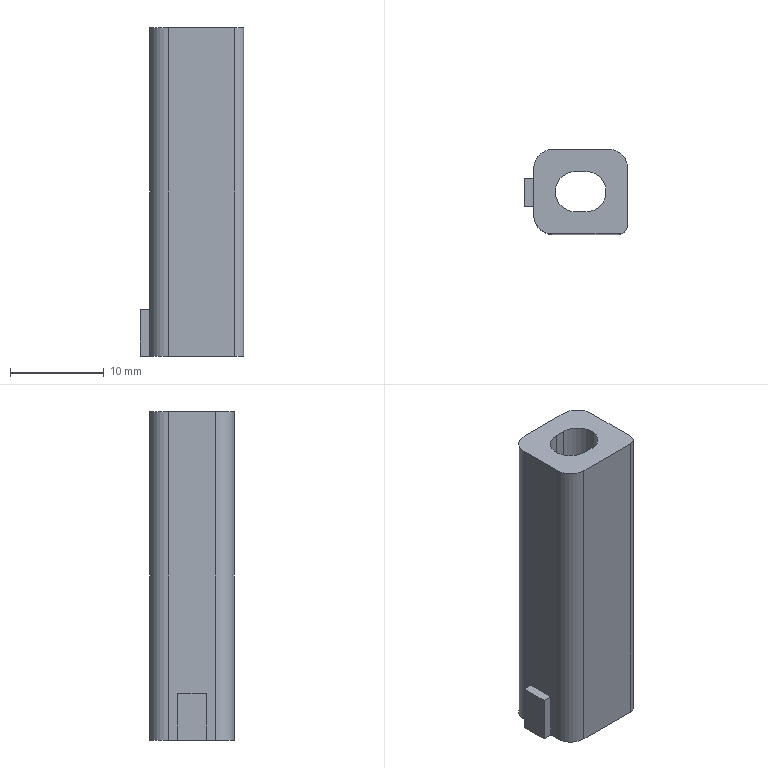Part | NX | features DIE-93 2 | 1 solid | 23 faces | box 11 x 9 x 35 mm | volume 2128 mm3 | plane 15 | cylinder 8 | commonest cylinder face diameters 4 x3 4.32 x2 5.32 x2 2 x1
STEP:
#1=CARTESIAN_POINT('',(4116.686,-879.282,853.716));
#2=VERTEX_POINT('',#1);
#3=CARTESIAN_POINT('',(4117.786,-879.282,853.716));
#4=VERTEX_POINT('',#3);
#5=CARTESIAN_POINT('',(4116.576,-879.282,853.716));
#6=DIRECTION('',(1.,0.,0.));
#7=VECTOR('',#6,1000.);
#8=LINE('',#5,#7);
#9=EDGE_CURVE('',#2,#4,#8,.T.);
#10=ORIENTED_EDGE('',*,*,#9,.F.);
#11=CARTESIAN_POINT('',(4116.686,-879.282,858.716));
#12=VERTEX_POINT('',#11);
#13=CARTESIAN_POINT('',(4116.686,-879.282,862.216));
#14=DIRECTION('',(0.,0.,-1.));
#15=VECTOR('',#14,1000.);
#16=LINE('',#13,#15);
#17=EDGE_CURVE('',#12,#2,#16,.T.);
#18=ORIENTED_EDGE('',*,*,#17,.F.);
#19=CARTESIAN_POINT('',(4117.786,-879.282,858.716));
#20=VERTEX_POINT('',#19);
#21=CARTESIAN_POINT('',(4123.586,-879.282,858.716));
#22=DIRECTION('',(-1.,0.,0.));
#23=VECTOR('',#22,1000.);
#24=LINE('',#21,#23);
#25=EDGE_CURVE('',#20,#12,#24,.T.);
#26=ORIENTED_EDGE('',*,*,#25,.F.);
#27=CARTESIAN_POINT('',(4117.786,-879.282,862.216));
#28=DIRECTION('',(0.,0.,-1.));
#29=VECTOR('',#28,1000.);
#30=LINE('',#27,#29);
#31=EDGE_CURVE('',#4,#20,#30,.F.);
#32=ORIENTED_EDGE('',*,*,#31,.F.);
#33=EDGE_LOOP('',(#10,#18,#26,#32));
#34=FACE_BOUND('',#33,.T.);
#35=CARTESIAN_POINT('',(4116.576,-879.282,870.016));
#36=DIRECTION('',(0.,1.,0.));
#37=DIRECTION('',(1.,0.,0.));
#38=AXIS2_PLACEMENT_3D('',#35,#36,#37);
#39=PLANE('',#38);
#40=ADVANCED_FACE('',(#34),#39,.T.);
#41=CARTESIAN_POINT('',(4117.786,-874.962,858.716));
#42=VERTEX_POINT('',#41);
#43=CARTESIAN_POINT('',(4117.786,-874.962,853.716));
#44=VERTEX_POINT('',#43);
#45=CARTESIAN_POINT('',(4117.786,-874.962,862.216));
#46=DIRECTION('',(0.,0.,-1.));
#47=VECTOR('',#46,1000.);
#48=LINE('',#45,#47);
#49=EDGE_CURVE('',#42,#44,#48,.T.);
#50=ORIENTED_EDGE('',*,*,#49,.T.);
#51=CARTESIAN_POINT('',(4117.786,-877.122,853.716));
#52=DIRECTION('',(0.,0.,1.));
#53=DIRECTION('',(1.,0.,0.));
#54=AXIS2_PLACEMENT_3D('',#51,#52,#53);
#55=CIRCLE('',#54,2.16);
#56=EDGE_CURVE('',#4,#44,#55,.T.);
#57=ORIENTED_EDGE('',*,*,#56,.F.);
#58=ORIENTED_EDGE('',*,*,#31,.T.);
#59=CARTESIAN_POINT('',(4117.786,-877.122,858.716));
#60=DIRECTION('',(0.,0.,1.));
#61=DIRECTION('',(1.,0.,0.));
#62=AXIS2_PLACEMENT_3D('',#59,#60,#61);
#63=CIRCLE('',#62,2.16);
#64=EDGE_CURVE('',#20,#42,#63,.T.);
#65=ORIENTED_EDGE('',*,*,#64,.T.);
#66=EDGE_LOOP('',(#50,#57,#58,#65));
#67=FACE_BOUND('',#66,.T.);
#68=CARTESIAN_POINT('',(4117.786,-877.122,862.216));
#69=DIRECTION('',(0.,0.,-1.));
#70=DIRECTION('',(-1.,0.,0.));
#71=AXIS2_PLACEMENT_3D('',#68,#69,#70);
#72=CYLINDRICAL_SURFACE('',#71,2.16);
#73=ADVANCED_FACE('',(#67),#72,.F.);
#74=CARTESIAN_POINT('',(4116.686,-874.962,853.716));
#75=VERTEX_POINT('',#74);
#76=CARTESIAN_POINT('',(4117.896,-874.962,853.716));
#77=DIRECTION('',(-1.,0.,0.));
#78=VECTOR('',#77,1000.);
#79=LINE('',#76,#78);
#80=EDGE_CURVE('',#44,#75,#79,.T.);
#81=ORIENTED_EDGE('',*,*,#80,.F.);
#82=ORIENTED_EDGE('',*,*,#49,.F.);
#83=CARTESIAN_POINT('',(4116.686,-874.962,858.716));
#84=VERTEX_POINT('',#83);
#85=CARTESIAN_POINT('',(4123.586,-874.962,858.716));
#86=DIRECTION('',(1.,0.,0.));
#87=VECTOR('',#86,1000.);
#88=LINE('',#85,#87);
#89=EDGE_CURVE('',#84,#42,#88,.T.);
#90=ORIENTED_EDGE('',*,*,#89,.F.);
#91=CARTESIAN_POINT('',(4116.686,-874.962,862.216));
#92=DIRECTION('',(0.,0.,-1.));
#93=VECTOR('',#92,1000.);
#94=LINE('',#91,#93);
#95=EDGE_CURVE('',#75,#84,#94,.F.);
#96=ORIENTED_EDGE('',*,*,#95,.F.);
#97=EDGE_LOOP('',(#81,#82,#90,#96));
#98=FACE_BOUND('',#97,.T.);
#99=CARTESIAN_POINT('',(4117.896,-874.962,870.016));
#100=DIRECTION('',(0.,-1.,0.));
#101=DIRECTION('',(-1.,0.,0.));
#102=AXIS2_PLACEMENT_3D('',#99,#100,#101);
#103=PLANE('',#102);
#104=ADVANCED_FACE('',(#98),#103,.T.);
#105=ORIENTED_EDGE('',*,*,#17,.T.);
#106=CARTESIAN_POINT('',(4116.686,-877.122,853.716));
#107=DIRECTION('',(0.,0.,1.));
#108=DIRECTION('',(1.,0.,0.));
#109=AXIS2_PLACEMENT_3D('',#106,#107,#108);
#110=CIRCLE('',#109,2.16);
#111=EDGE_CURVE('',#75,#2,#110,.T.);
#112=ORIENTED_EDGE('',*,*,#111,.F.);
#113=ORIENTED_EDGE('',*,*,#95,.T.);
#114=CARTESIAN_POINT('',(4116.686,-877.122,858.716));
#115=DIRECTION('',(0.,0.,1.));
#116=DIRECTION('',(1.,0.,0.));
#117=AXIS2_PLACEMENT_3D('',#114,#115,#116);
#118=CIRCLE('',#117,2.16);
#119=EDGE_CURVE('',#84,#12,#118,.T.);
#120=ORIENTED_EDGE('',*,*,#119,.T.);
#121=EDGE_LOOP('',(#105,#112,#113,#120));
#122=FACE_BOUND('',#121,.T.);
#123=CARTESIAN_POINT('',(4116.686,-877.122,862.216));
#124=DIRECTION('',(0.,0.,-1.));
#125=DIRECTION('',(1.,0.,0.));
#126=AXIS2_PLACEMENT_3D('',#123,#124,#125);
#127=CYLINDRICAL_SURFACE('',#126,2.16);
#128=ADVANCED_FACE('',(#122),#127,.F.);
#129=ORIENTED_EDGE('',*,*,#119,.F.);
#130=ORIENTED_EDGE('',*,*,#89,.T.);
#131=ORIENTED_EDGE('',*,*,#64,.F.);
#132=ORIENTED_EDGE('',*,*,#25,.T.);
#133=EDGE_LOOP('',(#129,#130,#131,#132));
#134=FACE_BOUND('',#133,.T.);
#135=CARTESIAN_POINT('',(4122.236,-874.622,858.716));
#136=VERTEX_POINT('',#135);
#137=CARTESIAN_POINT('',(4122.236,-880.622,858.716));
#138=VERTEX_POINT('',#137);
#139=CARTESIAN_POINT('',(4122.236,-877.122,858.716));
#140=DIRECTION('',(0.,-1.,0.));
#141=VECTOR('',#140,1000.);
#142=LINE('',#139,#141);
#143=EDGE_CURVE('',#136,#138,#142,.T.);
#144=ORIENTED_EDGE('',*,*,#143,.F.);
#145=CARTESIAN_POINT('',(4120.236,-872.622,858.716));
#146=VERTEX_POINT('',#145);
#147=CARTESIAN_POINT('',(4120.236,-874.622,858.716));
#148=DIRECTION('',(0.,0.,1.));
#149=DIRECTION('',(1.,0.,0.));
#150=AXIS2_PLACEMENT_3D('',#147,#148,#149);
#151=CIRCLE('',#150,2.);
#152=EDGE_CURVE('',#146,#136,#151,.F.);
#153=ORIENTED_EDGE('',*,*,#152,.F.);
#154=CARTESIAN_POINT('',(4114.236,-872.622,858.716));
#155=VERTEX_POINT('',#154);
#156=CARTESIAN_POINT('',(4117.236,-872.622,858.716));
#157=DIRECTION('',(1.,0.,0.));
#158=VECTOR('',#157,1000.);
#159=LINE('',#156,#158);
#160=EDGE_CURVE('',#155,#146,#159,.T.);
#161=ORIENTED_EDGE('',*,*,#160,.F.);
#162=CARTESIAN_POINT('',(4112.236,-874.622,858.716));
#163=VERTEX_POINT('',#162);
#164=CARTESIAN_POINT('',(4114.236,-874.622,858.716));
#165=DIRECTION('',(0.,0.,1.));
#166=DIRECTION('',(1.,0.,0.));
#167=AXIS2_PLACEMENT_3D('',#164,#165,#166);
#168=CIRCLE('',#167,2.);
#169=EDGE_CURVE('',#155,#163,#168,.T.);
#170=ORIENTED_EDGE('',*,*,#169,.T.);
#171=CARTESIAN_POINT('',(4112.236,-879.622,858.716));
#172=VERTEX_POINT('',#171);
#173=CARTESIAN_POINT('',(4112.236,-877.122,858.716));
#174=DIRECTION('',(0.,1.,0.));
#175=VECTOR('',#174,1000.);
#176=LINE('',#173,#175);
#177=EDGE_CURVE('',#172,#163,#176,.T.);
#178=ORIENTED_EDGE('',*,*,#177,.F.);
#179=CARTESIAN_POINT('',(4114.236,-881.622,858.716));
#180=VERTEX_POINT('',#179);
#181=CARTESIAN_POINT('',(4114.236,-879.622,858.716));
#182=DIRECTION('',(0.,0.,1.));
#183=DIRECTION('',(1.,0.,0.));
#184=AXIS2_PLACEMENT_3D('',#181,#182,#183);
#185=CIRCLE('',#184,2.);
#186=EDGE_CURVE('',#172,#180,#185,.T.);
#187=ORIENTED_EDGE('',*,*,#186,.T.);
#188=CARTESIAN_POINT('',(4121.236,-881.622,858.716));
#189=VERTEX_POINT('',#188);
#190=CARTESIAN_POINT('',(4117.236,-881.622,858.716));
#191=DIRECTION('',(-1.,0.,0.));
#192=VECTOR('',#191,1000.);
#193=LINE('',#190,#192);
#194=EDGE_CURVE('',#189,#180,#193,.T.);
#195=ORIENTED_EDGE('',*,*,#194,.F.);
#196=CARTESIAN_POINT('',(4121.236,-880.622,858.716));
#197=DIRECTION('',(0.,0.,1.));
#198=DIRECTION('',(1.,0.,0.));
#199=AXIS2_PLACEMENT_3D('',#196,#197,#198);
#200=CIRCLE('',#199,1.);
#201=EDGE_CURVE('',#138,#189,#200,.F.);
#202=ORIENTED_EDGE('',*,*,#201,.F.);
#203=EDGE_LOOP('',(#144,#153,#161,#170,#178,#187,#195,#202));
#204=FACE_BOUND('',#203,.T.);
#205=CARTESIAN_POINT('',(4123.586,-858.122,858.716));
#206=DIRECTION('',(0.,0.,1.));
#207=DIRECTION('',(-1.,0.,0.));
#208=AXIS2_PLACEMENT_3D('',#205,#206,#207);
#209=PLANE('',#208);
#210=ADVANCED_FACE('',(#134,#204),#209,.T.);
#211=ORIENTED_EDGE('',*,*,#9,.T.);
#212=ORIENTED_EDGE('',*,*,#56,.T.);
#213=ORIENTED_EDGE('',*,*,#80,.T.);
#214=ORIENTED_EDGE('',*,*,#111,.T.);
#215=EDGE_LOOP('',(#211,#212,#213,#214));
#216=FACE_BOUND('',#215,.T.);
#217=CARTESIAN_POINT('',(4117.786,-879.782,853.716));
#218=VERTEX_POINT('',#217);
#219=CARTESIAN_POINT('',(4116.686,-879.782,853.716));
#220=VERTEX_POINT('',#219);
#221=CARTESIAN_POINT('',(4079.736,-879.782,853.716));
#222=DIRECTION('',(-1.,0.,0.));
#223=VECTOR('',#222,1000.);
#224=LINE('',#221,#223);
#225=EDGE_CURVE('',#218,#220,#224,.T.);
#226=ORIENTED_EDGE('',*,*,#225,.T.);
#227=CARTESIAN_POINT('',(4116.686,-874.462,853.716));
#228=VERTEX_POINT('',#227);
#229=CARTESIAN_POINT('',(4116.686,-877.122,853.716));
#230=DIRECTION('',(0.,0.,1.));
#231=DIRECTION('',(1.,0.,0.));
#232=AXIS2_PLACEMENT_3D('',#229,#230,#231);
#233=CIRCLE('',#232,2.66);
#234=EDGE_CURVE('',#220,#228,#233,.F.);
#235=ORIENTED_EDGE('',*,*,#234,.T.);
#236=CARTESIAN_POINT('',(4117.786,-874.462,853.716));
#237=VERTEX_POINT('',#236);
#238=CARTESIAN_POINT('',(4079.736,-874.462,853.716));
#239=DIRECTION('',(1.,0.,0.));
#240=VECTOR('',#239,1000.);
#241=LINE('',#238,#240);
#242=EDGE_CURVE('',#228,#237,#241,.T.);
#243=ORIENTED_EDGE('',*,*,#242,.T.);
#244=CARTESIAN_POINT('',(4117.786,-877.122,853.716));
#245=DIRECTION('',(0.,0.,1.));
#246=DIRECTION('',(1.,0.,0.));
#247=AXIS2_PLACEMENT_3D('',#244,#245,#246);
#248=CIRCLE('',#247,2.66);
#249=EDGE_CURVE('',#237,#218,#248,.F.);
#250=ORIENTED_EDGE('',*,*,#249,.T.);
#251=EDGE_LOOP('',(#226,#235,#243,#250));
#252=FACE_BOUND('',#251,.T.);
#253=CARTESIAN_POINT('',(4079.736,-858.122,853.716));
#254=DIRECTION('',(0.,0.,1.));
#255=DIRECTION('',(1.,0.,0.));
#256=AXIS2_PLACEMENT_3D('',#253,#254,#255);
#257=PLANE('',#256);
#258=ADVANCED_FACE('',(#216,#252),#257,.F.);
#259=CARTESIAN_POINT('',(4117.786,-879.782,823.716));
#260=VERTEX_POINT('',#259);
#261=CARTESIAN_POINT('',(4117.786,-874.462,823.716));
#262=VERTEX_POINT('',#261);
#263=CARTESIAN_POINT('',(4117.786,-877.122,823.716));
#264=DIRECTION('',(0.,0.,-1.));
#265=DIRECTION('',(-1.,0.,0.));
#266=AXIS2_PLACEMENT_3D('',#263,#264,#265);
#267=CIRCLE('',#266,2.66);
#268=EDGE_CURVE('',#260,#262,#267,.F.);
#269=ORIENTED_EDGE('',*,*,#268,.F.);
#270=CARTESIAN_POINT('',(4117.786,-879.782,862.216));
#271=DIRECTION('',(0.,0.,-1.));
#272=VECTOR('',#271,1000.);
#273=LINE('',#270,#272);
#274=EDGE_CURVE('',#260,#218,#273,.F.);
#275=ORIENTED_EDGE('',*,*,#274,.T.);
#276=ORIENTED_EDGE('',*,*,#249,.F.);
#277=CARTESIAN_POINT('',(4117.786,-874.462,862.216));
#278=DIRECTION('',(0.,0.,-1.));
#279=VECTOR('',#278,1000.);
#280=LINE('',#277,#279);
#281=EDGE_CURVE('',#237,#262,#280,.T.);
#282=ORIENTED_EDGE('',*,*,#281,.T.);
#283=EDGE_LOOP('',(#269,#275,#276,#282));
#284=FACE_BOUND('',#283,.T.);
#285=CARTESIAN_POINT('',(4117.786,-877.122,862.216));
#286=DIRECTION('',(0.,0.,-1.));
#287=DIRECTION('',(-1.,0.,0.));
#288=AXIS2_PLACEMENT_3D('',#285,#286,#287);
#289=CYLINDRICAL_SURFACE('',#288,2.66);
#290=ADVANCED_FACE('',(#284),#289,.F.);
#291=ORIENTED_EDGE('',*,*,#274,.F.);
#292=CARTESIAN_POINT('',(4116.686,-879.782,823.716));
#293=VERTEX_POINT('',#292);
#294=CARTESIAN_POINT('',(4123.586,-879.782,823.716));
#295=DIRECTION('',(1.,0.,0.));
#296=VECTOR('',#295,1000.);
#297=LINE('',#294,#296);
#298=EDGE_CURVE('',#293,#260,#297,.T.);
#299=ORIENTED_EDGE('',*,*,#298,.F.);
#300=CARTESIAN_POINT('',(4116.686,-879.782,862.216));
#301=DIRECTION('',(0.,0.,-1.));
#302=VECTOR('',#301,1000.);
#303=LINE('',#300,#302);
#304=EDGE_CURVE('',#220,#293,#303,.T.);
#305=ORIENTED_EDGE('',*,*,#304,.F.);
#306=ORIENTED_EDGE('',*,*,#225,.F.);
#307=EDGE_LOOP('',(#291,#299,#305,#306));
#308=FACE_BOUND('',#307,.T.);
#309=CARTESIAN_POINT('',(4116.576,-879.782,870.016));
#310=DIRECTION('',(0.,1.,0.));
#311=DIRECTION('',(1.,0.,0.));
#312=AXIS2_PLACEMENT_3D('',#309,#310,#311);
#313=PLANE('',#312);
#314=ADVANCED_FACE('',(#308),#313,.T.);
#315=CARTESIAN_POINT('',(4116.686,-874.462,823.716));
#316=VERTEX_POINT('',#315);
#317=CARTESIAN_POINT('',(4116.686,-877.122,823.716));
#318=DIRECTION('',(0.,0.,-1.));
#319=DIRECTION('',(-1.,0.,0.));
#320=AXIS2_PLACEMENT_3D('',#317,#318,#319);
#321=CIRCLE('',#320,2.66);
#322=EDGE_CURVE('',#316,#293,#321,.F.);
#323=ORIENTED_EDGE('',*,*,#322,.F.);
#324=CARTESIAN_POINT('',(4116.686,-874.462,862.216));
#325=DIRECTION('',(0.,0.,-1.));
#326=VECTOR('',#325,1000.);
#327=LINE('',#324,#326);
#328=EDGE_CURVE('',#316,#228,#327,.F.);
#329=ORIENTED_EDGE('',*,*,#328,.T.);
#330=ORIENTED_EDGE('',*,*,#234,.F.);
#331=ORIENTED_EDGE('',*,*,#304,.T.);
#332=EDGE_LOOP('',(#323,#329,#330,#331));
#333=FACE_BOUND('',#332,.T.);
#334=CARTESIAN_POINT('',(4116.686,-877.122,862.216));
#335=DIRECTION('',(0.,0.,-1.));
#336=DIRECTION('',(1.,0.,0.));
#337=AXIS2_PLACEMENT_3D('',#334,#335,#336);
#338=CYLINDRICAL_SURFACE('',#337,2.66);
#339=ADVANCED_FACE('',(#333),#338,.F.);
#340=ORIENTED_EDGE('',*,*,#328,.F.);
#341=CARTESIAN_POINT('',(4123.586,-874.462,823.716));
#342=DIRECTION('',(-1.,0.,0.));
#343=VECTOR('',#342,1000.);
#344=LINE('',#341,#343);
#345=EDGE_CURVE('',#262,#316,#344,.T.);
#346=ORIENTED_EDGE('',*,*,#345,.F.);
#347=ORIENTED_EDGE('',*,*,#281,.F.);
#348=ORIENTED_EDGE('',*,*,#242,.F.);
#349=EDGE_LOOP('',(#340,#346,#347,#348));
#350=FACE_BOUND('',#349,.T.);
#351=CARTESIAN_POINT('',(4117.896,-874.462,870.016));
#352=DIRECTION('',(0.,-1.,0.));
#353=DIRECTION('',(-1.,0.,0.));
#354=AXIS2_PLACEMENT_3D('',#351,#352,#353);
#355=PLANE('',#354);
#356=ADVANCED_FACE('',(#350),#355,.T.);
#357=CARTESIAN_POINT('',(4112.236,-878.622,823.716));
#358=VERTEX_POINT('',#357);
#359=CARTESIAN_POINT('',(4112.236,-879.622,823.716));
#360=VERTEX_POINT('',#359);
#361=CARTESIAN_POINT('',(4112.236,-877.122,823.716));
#362=DIRECTION('',(0.,-1.,0.));
#363=VECTOR('',#362,1000.);
#364=LINE('',#361,#363);
#365=EDGE_CURVE('',#358,#360,#364,.T.);
#366=ORIENTED_EDGE('',*,*,#365,.F.);
#367=CARTESIAN_POINT('',(4111.236,-878.622,823.716));
#368=VERTEX_POINT('',#367);
#369=CARTESIAN_POINT('',(0.,-878.622,823.716));
#370=DIRECTION('',(-1.,0.,0.));
#371=VECTOR('',#370,1000.);
#372=LINE('',#369,#371);
#373=EDGE_CURVE('',#358,#368,#372,.T.);
#374=ORIENTED_EDGE('',*,*,#373,.T.);
#375=CARTESIAN_POINT('',(4111.236,-875.622,823.716));
#376=VERTEX_POINT('',#375);
#377=CARTESIAN_POINT('',(4111.236,-879.622,823.716));
#378=DIRECTION('',(0.,1.,0.));
#379=VECTOR('',#378,1000.);
#380=LINE('',#377,#379);
#381=EDGE_CURVE('',#368,#376,#380,.T.);
#382=ORIENTED_EDGE('',*,*,#381,.T.);
#383=CARTESIAN_POINT('',(4112.236,-875.622,823.716));
#384=VERTEX_POINT('',#383);
#385=CARTESIAN_POINT('',(0.,-875.622,823.716));
#386=DIRECTION('',(1.,0.,0.));
#387=VECTOR('',#386,1000.);
#388=LINE('',#385,#387);
#389=EDGE_CURVE('',#376,#384,#388,.T.);
#390=ORIENTED_EDGE('',*,*,#389,.T.);
#391=CARTESIAN_POINT('',(4112.236,-874.622,823.716));
#392=VERTEX_POINT('',#391);
#393=CARTESIAN_POINT('',(4112.236,-877.122,823.716));
#394=DIRECTION('',(0.,-1.,0.));
#395=VECTOR('',#394,1000.);
#396=LINE('',#393,#395);
#397=EDGE_CURVE('',#392,#384,#396,.T.);
#398=ORIENTED_EDGE('',*,*,#397,.F.);
#399=CARTESIAN_POINT('',(4114.236,-872.622,823.716));
#400=VERTEX_POINT('',#399);
#401=CARTESIAN_POINT('',(4114.236,-874.622,823.716));
#402=DIRECTION('',(0.,0.,-1.));
#403=DIRECTION('',(-1.,0.,0.));
#404=AXIS2_PLACEMENT_3D('',#401,#402,#403);
#405=CIRCLE('',#404,2.);
#406=EDGE_CURVE('',#400,#392,#405,.F.);
#407=ORIENTED_EDGE('',*,*,#406,.F.);
#408=CARTESIAN_POINT('',(4120.236,-872.622,823.716));
#409=VERTEX_POINT('',#408);
#410=CARTESIAN_POINT('',(4117.236,-872.622,823.716));
#411=DIRECTION('',(-1.,0.,0.));
#412=VECTOR('',#411,1000.);
#413=LINE('',#410,#412);
#414=EDGE_CURVE('',#409,#400,#413,.T.);
#415=ORIENTED_EDGE('',*,*,#414,.F.);
#416=CARTESIAN_POINT('',(4122.236,-874.622,823.716));
#417=VERTEX_POINT('',#416);
#418=CARTESIAN_POINT('',(4120.236,-874.622,823.716));
#419=DIRECTION('',(0.,0.,-1.));
#420=DIRECTION('',(-1.,0.,0.));
#421=AXIS2_PLACEMENT_3D('',#418,#419,#420);
#422=CIRCLE('',#421,2.);
#423=EDGE_CURVE('',#417,#409,#422,.F.);
#424=ORIENTED_EDGE('',*,*,#423,.F.);
#425=CARTESIAN_POINT('',(4122.236,-880.622,823.716));
#426=VERTEX_POINT('',#425);
#427=CARTESIAN_POINT('',(4122.236,-877.122,823.716));
#428=DIRECTION('',(0.,1.,0.));
#429=VECTOR('',#428,1000.);
#430=LINE('',#427,#429);
#431=EDGE_CURVE('',#426,#417,#430,.T.);
#432=ORIENTED_EDGE('',*,*,#431,.F.);
#433=CARTESIAN_POINT('',(4121.236,-881.622,823.716));
#434=VERTEX_POINT('',#433);
#435=CARTESIAN_POINT('',(4121.236,-880.622,823.716));
#436=DIRECTION('',(0.,0.,-1.));
#437=DIRECTION('',(-1.,0.,0.));
#438=AXIS2_PLACEMENT_3D('',#435,#436,#437);
#439=CIRCLE('',#438,1.);
#440=EDGE_CURVE('',#426,#434,#439,.T.);
#441=ORIENTED_EDGE('',*,*,#440,.T.);
#442=CARTESIAN_POINT('',(4114.236,-881.622,823.716));
#443=VERTEX_POINT('',#442);
#444=CARTESIAN_POINT('',(4117.236,-881.622,823.716));
#445=DIRECTION('',(1.,0.,0.));
#446=VECTOR('',#445,1000.);
#447=LINE('',#444,#446);
#448=EDGE_CURVE('',#434,#443,#447,.F.);
#449=ORIENTED_EDGE('',*,*,#448,.T.);
#450=CARTESIAN_POINT('',(4114.236,-879.622,823.716));
#451=DIRECTION('',(0.,0.,-1.));
#452=DIRECTION('',(-1.,0.,0.));
#453=AXIS2_PLACEMENT_3D('',#450,#451,#452);
#454=CIRCLE('',#453,2.);
#455=EDGE_CURVE('',#360,#443,#454,.F.);
#456=ORIENTED_EDGE('',*,*,#455,.F.);
#457=EDGE_LOOP('',(#366,#374,#382,#390,#398,#407,#415,#424,#432,#441,#449,#456));
#458=FACE_BOUND('',#457,.T.);
#459=ORIENTED_EDGE('',*,*,#345,.T.);
#460=ORIENTED_EDGE('',*,*,#322,.T.);
#461=ORIENTED_EDGE('',*,*,#298,.T.);
#462=ORIENTED_EDGE('',*,*,#268,.T.);
#463=EDGE_LOOP('',(#459,#460,#461,#462));
#464=FACE_BOUND('',#463,.T.);
#465=CARTESIAN_POINT('',(4123.586,-858.122,823.716));
#466=DIRECTION('',(0.,0.,-1.));
#467=DIRECTION('',(-1.,0.,0.));
#468=AXIS2_PLACEMENT_3D('',#465,#466,#467);
#469=PLANE('',#468);
#470=ADVANCED_FACE('',(#458,#464),#469,.T.);
#471=ORIENTED_EDGE('',*,*,#414,.T.);
#472=CARTESIAN_POINT('',(4114.236,-872.622,823.716));
#473=DIRECTION('',(0.,0.,1.));
#474=VECTOR('',#473,1000.);
#475=LINE('',#472,#474);
#476=EDGE_CURVE('',#400,#155,#475,.T.);
#477=ORIENTED_EDGE('',*,*,#476,.T.);
#478=ORIENTED_EDGE('',*,*,#160,.T.);
#479=CARTESIAN_POINT('',(4120.236,-872.622,823.716));
#480=DIRECTION('',(0.,0.,1.));
#481=VECTOR('',#480,1000.);
#482=LINE('',#479,#481);
#483=EDGE_CURVE('',#146,#409,#482,.F.);
#484=ORIENTED_EDGE('',*,*,#483,.T.);
#485=EDGE_LOOP('',(#471,#477,#478,#484));
#486=FACE_BOUND('',#485,.T.);
#487=CARTESIAN_POINT('',(4117.236,-872.622,823.716));
#488=DIRECTION('',(0.,1.,0.));
#489=DIRECTION('',(0.,0.,-1.));
#490=AXIS2_PLACEMENT_3D('',#487,#488,#489);
#491=PLANE('',#490);
#492=ADVANCED_FACE('',(#486),#491,.T.);
#493=ORIENTED_EDGE('',*,*,#143,.T.);
#494=CARTESIAN_POINT('',(4122.236,-880.622,823.716));
#495=DIRECTION('',(0.,0.,1.));
#496=VECTOR('',#495,1000.);
#497=LINE('',#494,#496);
#498=EDGE_CURVE('',#138,#426,#497,.F.);
#499=ORIENTED_EDGE('',*,*,#498,.T.);
#500=ORIENTED_EDGE('',*,*,#431,.T.);
#501=CARTESIAN_POINT('',(4122.236,-874.622,823.716));
#502=DIRECTION('',(0.,0.,1.));
#503=VECTOR('',#502,1000.);
#504=LINE('',#501,#503);
#505=EDGE_CURVE('',#417,#136,#504,.T.);
#506=ORIENTED_EDGE('',*,*,#505,.T.);
#507=EDGE_LOOP('',(#493,#499,#500,#506));
#508=FACE_BOUND('',#507,.T.);
#509=CARTESIAN_POINT('',(4122.236,-877.122,823.716));
#510=DIRECTION('',(1.,0.,0.));
#511=DIRECTION('',(0.,0.,1.));
#512=AXIS2_PLACEMENT_3D('',#509,#510,#511);
#513=PLANE('',#512);
#514=ADVANCED_FACE('',(#508),#513,.T.);
#515=ORIENTED_EDGE('',*,*,#448,.F.);
#516=CARTESIAN_POINT('',(4121.236,-881.622,823.716));
#517=DIRECTION('',(0.,0.,1.));
#518=VECTOR('',#517,1000.);
#519=LINE('',#516,#518);
#520=EDGE_CURVE('',#434,#189,#519,.T.);
#521=ORIENTED_EDGE('',*,*,#520,.T.);
#522=ORIENTED_EDGE('',*,*,#194,.T.);
#523=CARTESIAN_POINT('',(4114.236,-881.622,823.716));
#524=DIRECTION('',(0.,0.,1.));
#525=VECTOR('',#524,1000.);
#526=LINE('',#523,#525);
#527=EDGE_CURVE('',#180,#443,#526,.F.);
#528=ORIENTED_EDGE('',*,*,#527,.T.);
#529=EDGE_LOOP('',(#515,#521,#522,#528));
#530=FACE_BOUND('',#529,.T.);
#531=CARTESIAN_POINT('',(4117.236,-881.622,823.716));
#532=DIRECTION('',(0.,-1.,0.));
#533=DIRECTION('',(0.,0.,1.));
#534=AXIS2_PLACEMENT_3D('',#531,#532,#533);
#535=PLANE('',#534);
#536=ADVANCED_FACE('',(#530),#535,.T.);
#537=CARTESIAN_POINT('',(4112.236,-875.622,828.716));
#538=VERTEX_POINT('',#537);
#539=CARTESIAN_POINT('',(4112.236,-875.622,823.716));
#540=DIRECTION('',(0.,0.,-1.));
#541=VECTOR('',#540,1000.);
#542=LINE('',#539,#541);
#543=EDGE_CURVE('',#538,#384,#542,.T.);
#544=ORIENTED_EDGE('',*,*,#543,.F.);
#545=CARTESIAN_POINT('',(4112.236,-878.622,828.716));
#546=VERTEX_POINT('',#545);
#547=CARTESIAN_POINT('',(4112.236,-877.122,828.716));
#548=DIRECTION('',(0.,-1.,0.));
#549=VECTOR('',#548,1000.);
#550=LINE('',#547,#549);
#551=EDGE_CURVE('',#538,#546,#550,.T.);
#552=ORIENTED_EDGE('',*,*,#551,.T.);
#553=CARTESIAN_POINT('',(4112.236,-878.622,823.716));
#554=DIRECTION('',(0.,0.,1.));
#555=VECTOR('',#554,1000.);
#556=LINE('',#553,#555);
#557=EDGE_CURVE('',#358,#546,#556,.T.);
#558=ORIENTED_EDGE('',*,*,#557,.F.);
#559=ORIENTED_EDGE('',*,*,#365,.T.);
#560=CARTESIAN_POINT('',(4112.236,-879.622,823.716));
#561=DIRECTION('',(0.,0.,1.));
#562=VECTOR('',#561,1000.);
#563=LINE('',#560,#562);
#564=EDGE_CURVE('',#360,#172,#563,.T.);
#565=ORIENTED_EDGE('',*,*,#564,.T.);
#566=ORIENTED_EDGE('',*,*,#177,.T.);
#567=CARTESIAN_POINT('',(4112.236,-874.622,823.716));
#568=DIRECTION('',(0.,0.,1.));
#569=VECTOR('',#568,1000.);
#570=LINE('',#567,#569);
#571=EDGE_CURVE('',#163,#392,#570,.F.);
#572=ORIENTED_EDGE('',*,*,#571,.T.);
#573=ORIENTED_EDGE('',*,*,#397,.T.);
#574=EDGE_LOOP('',(#544,#552,#558,#559,#565,#566,#572,#573));
#575=FACE_BOUND('',#574,.T.);
#576=CARTESIAN_POINT('',(4112.236,-877.122,823.716));
#577=DIRECTION('',(-1.,0.,0.));
#578=DIRECTION('',(0.,0.,-1.));
#579=AXIS2_PLACEMENT_3D('',#576,#577,#578);
#580=PLANE('',#579);
#581=ADVANCED_FACE('',(#575),#580,.T.);
#582=ORIENTED_EDGE('',*,*,#455,.T.);
#583=ORIENTED_EDGE('',*,*,#527,.F.);
#584=ORIENTED_EDGE('',*,*,#186,.F.);
#585=ORIENTED_EDGE('',*,*,#564,.F.);
#586=EDGE_LOOP('',(#582,#583,#584,#585));
#587=FACE_BOUND('',#586,.T.);
#588=CARTESIAN_POINT('',(4114.236,-879.622,823.716));
#589=DIRECTION('',(0.,0.,1.));
#590=DIRECTION('',(1.,0.,0.));
#591=AXIS2_PLACEMENT_3D('',#588,#589,#590);
#592=CYLINDRICAL_SURFACE('',#591,2.);
#593=ADVANCED_FACE('',(#587),#592,.T.);
#594=ORIENTED_EDGE('',*,*,#406,.T.);
#595=ORIENTED_EDGE('',*,*,#571,.F.);
#596=ORIENTED_EDGE('',*,*,#169,.F.);
#597=ORIENTED_EDGE('',*,*,#476,.F.);
#598=EDGE_LOOP('',(#594,#595,#596,#597));
#599=FACE_BOUND('',#598,.T.);
#600=CARTESIAN_POINT('',(4114.236,-874.622,823.716));
#601=DIRECTION('',(0.,0.,1.));
#602=DIRECTION('',(1.,0.,0.));
#603=AXIS2_PLACEMENT_3D('',#600,#601,#602);
#604=CYLINDRICAL_SURFACE('',#603,2.);
#605=ADVANCED_FACE('',(#599),#604,.T.);
#606=ORIENTED_EDGE('',*,*,#423,.T.);
#607=ORIENTED_EDGE('',*,*,#483,.F.);
#608=ORIENTED_EDGE('',*,*,#152,.T.);
#609=ORIENTED_EDGE('',*,*,#505,.F.);
#610=EDGE_LOOP('',(#606,#607,#608,#609));
#611=FACE_BOUND('',#610,.T.);
#612=CARTESIAN_POINT('',(4120.236,-874.622,823.716));
#613=DIRECTION('',(0.,0.,1.));
#614=DIRECTION('',(1.,0.,0.));
#615=AXIS2_PLACEMENT_3D('',#612,#613,#614);
#616=CYLINDRICAL_SURFACE('',#615,2.);
#617=ADVANCED_FACE('',(#611),#616,.T.);
#618=ORIENTED_EDGE('',*,*,#440,.F.);
#619=ORIENTED_EDGE('',*,*,#498,.F.);
#620=ORIENTED_EDGE('',*,*,#201,.T.);
#621=ORIENTED_EDGE('',*,*,#520,.F.);
#622=EDGE_LOOP('',(#618,#619,#620,#621));
#623=FACE_BOUND('',#622,.T.);
#624=CARTESIAN_POINT('',(4121.236,-880.622,823.716));
#625=DIRECTION('',(0.,0.,1.));
#626=DIRECTION('',(1.,0.,0.));
#627=AXIS2_PLACEMENT_3D('',#624,#625,#626);
#628=CYLINDRICAL_SURFACE('',#627,1.);
#629=ADVANCED_FACE('',(#623),#628,.T.);
#630=CARTESIAN_POINT('',(4111.236,-875.622,828.716));
#631=VERTEX_POINT('',#630);
#632=CARTESIAN_POINT('',(0.,-875.622,828.716));
#633=DIRECTION('',(1.,0.,0.));
#634=VECTOR('',#633,1000.);
#635=LINE('',#632,#634);
#636=EDGE_CURVE('',#631,#538,#635,.T.);
#637=ORIENTED_EDGE('',*,*,#636,.T.);
#638=ORIENTED_EDGE('',*,*,#543,.T.);
#639=ORIENTED_EDGE('',*,*,#389,.F.);
#640=CARTESIAN_POINT('',(4111.236,-875.622,828.716));
#641=DIRECTION('',(0.,0.,-1.));
#642=VECTOR('',#641,1000.);
#643=LINE('',#640,#642);
#644=EDGE_CURVE('',#631,#376,#643,.T.);
#645=ORIENTED_EDGE('',*,*,#644,.F.);
#646=EDGE_LOOP('',(#637,#638,#639,#645));
#647=FACE_BOUND('',#646,.T.);
#648=CARTESIAN_POINT('',(4111.236,-875.622,828.716));
#649=DIRECTION('',(0.,1.,0.));
#650=DIRECTION('',(0.,0.,1.));
#651=AXIS2_PLACEMENT_3D('',#648,#649,#650);
#652=PLANE('',#651);
#653=ADVANCED_FACE('',(#647),#652,.T.);
#654=ORIENTED_EDGE('',*,*,#373,.F.);
#655=ORIENTED_EDGE('',*,*,#557,.T.);
#656=CARTESIAN_POINT('',(4111.236,-878.622,828.716));
#657=VERTEX_POINT('',#656);
#658=CARTESIAN_POINT('',(0.,-878.622,828.716));
#659=DIRECTION('',(-1.,0.,0.));
#660=VECTOR('',#659,1000.);
#661=LINE('',#658,#660);
#662=EDGE_CURVE('',#546,#657,#661,.T.);
#663=ORIENTED_EDGE('',*,*,#662,.T.);
#664=CARTESIAN_POINT('',(4111.236,-878.622,828.716));
#665=DIRECTION('',(0.,0.,-1.));
#666=VECTOR('',#665,1000.);
#667=LINE('',#664,#666);
#668=EDGE_CURVE('',#657,#368,#667,.T.);
#669=ORIENTED_EDGE('',*,*,#668,.T.);
#670=EDGE_LOOP('',(#654,#655,#663,#669));
#671=FACE_BOUND('',#670,.T.);
#672=CARTESIAN_POINT('',(4112.286,-878.622,828.716));
#673=DIRECTION('',(0.,-1.,0.));
#674=DIRECTION('',(0.,0.,-1.));
#675=AXIS2_PLACEMENT_3D('',#672,#673,#674);
#676=PLANE('',#675);
#677=ADVANCED_FACE('',(#671),#676,.T.);
#678=ORIENTED_EDGE('',*,*,#381,.F.);
#679=ORIENTED_EDGE('',*,*,#668,.F.);
#680=CARTESIAN_POINT('',(4111.236,-879.622,828.716));
#681=DIRECTION('',(0.,1.,0.));
#682=VECTOR('',#681,1000.);
#683=LINE('',#680,#682);
#684=EDGE_CURVE('',#657,#631,#683,.T.);
#685=ORIENTED_EDGE('',*,*,#684,.T.);
#686=ORIENTED_EDGE('',*,*,#644,.T.);
#687=EDGE_LOOP('',(#678,#679,#685,#686));
#688=FACE_BOUND('',#687,.T.);
#689=CARTESIAN_POINT('',(4111.236,-879.622,828.716));
#690=DIRECTION('',(-1.,0.,0.));
#691=DIRECTION('',(0.,0.,1.));
#692=AXIS2_PLACEMENT_3D('',#689,#690,#691);
#693=PLANE('',#692);
#694=ADVANCED_FACE('',(#688),#693,.T.);
#695=ORIENTED_EDGE('',*,*,#551,.F.);
#696=ORIENTED_EDGE('',*,*,#636,.F.);
#697=ORIENTED_EDGE('',*,*,#684,.F.);
#698=ORIENTED_EDGE('',*,*,#662,.F.);
#699=EDGE_LOOP('',(#695,#696,#697,#698));
#700=FACE_BOUND('',#699,.T.);
#701=CARTESIAN_POINT('',(0.,0.,828.716));
#702=DIRECTION('',(0.,0.,-1.));
#703=DIRECTION('',(-1.,0.,0.));
#704=AXIS2_PLACEMENT_3D('',#701,#702,#703);
#705=PLANE('',#704);
#706=ADVANCED_FACE('',(#700),#705,.F.);
#707=CLOSED_SHELL('',(#40,#73,#104,#128,#210,#258,#290,#314,#339,#356,#470,#492,#514,#536,#581,#593,#605,#617,#629,#653,#677,#694,#706));
#708=MANIFOLD_SOLID_BREP('',#707);
#709=(LENGTH_UNIT()NAMED_UNIT(*)SI_UNIT(.MILLI.,.METRE.));
#710=UNCERTAINTY_MEASURE_WITH_UNIT(LENGTH_MEASURE(0.00001),#709,'','');
#711=(NAMED_UNIT(*)PLANE_ANGLE_UNIT()SI_UNIT($,.RADIAN.));
#712=(NAMED_UNIT(*)SI_UNIT($,.STERADIAN.)SOLID_ANGLE_UNIT());
#713=(GEOMETRIC_REPRESENTATION_CONTEXT(3)GLOBAL_UNCERTAINTY_ASSIGNED_CONTEXT((#710))GLOBAL_UNIT_ASSIGNED_CONTEXT((#709,#711,#712))REPRESENTATION_CONTEXT('',''));
#714=ADVANCED_BREP_SHAPE_REPRESENTATION('',(#708),#713);